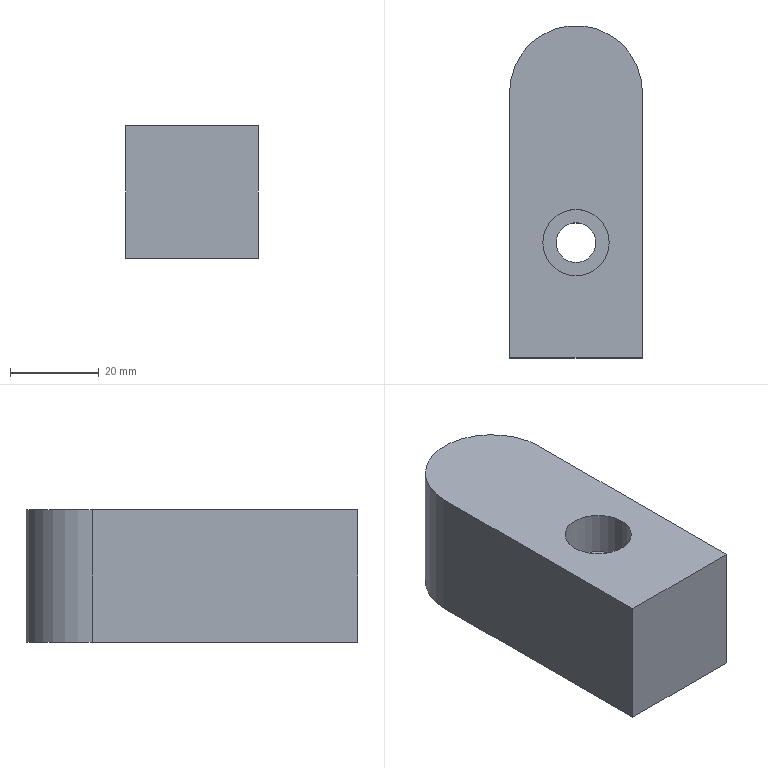Part | STEP file | 400v80 Tailstock Locating Pin | 1 solid | 11 faces | box 30 x 75 x 30 mm | volume 61563 mm3 | plane 6 | cylinder 5 | commonest cylinder face diameters 9 x2 15 x2 30 x1
STEP:
#1=CARTESIAN_POINT('',(-10.246,-122.222,0.));
#2=VERTEX_POINT('',#1);
#3=CARTESIAN_POINT('',(-19.246,-122.222,0.));
#4=VERTEX_POINT('',#3);
#5=CARTESIAN_POINT('',(-14.746,-122.222,0.));
#6=DIRECTION('',(0.,0.,-1.));
#7=DIRECTION('',(1.,0.,0.));
#8=AXIS2_PLACEMENT_3D('',#5,#6,#7);
#9=CIRCLE('',#8,4.5);
#10=EDGE_CURVE('',#2,#4,#9,.T.);
#11=ORIENTED_EDGE('',*,*,#10,.T.);
#12=CARTESIAN_POINT('',(-19.246,-122.222,20.));
#13=VERTEX_POINT('',#12);
#14=CARTESIAN_POINT('',(-19.246,-122.222,0.));
#15=DIRECTION('',(0.,0.,1.));
#16=VECTOR('',#15,1000.);
#17=LINE('',#14,#16);
#18=EDGE_CURVE('',#4,#13,#17,.T.);
#19=ORIENTED_EDGE('',*,*,#18,.T.);
#20=CARTESIAN_POINT('',(-10.246,-122.222,20.));
#21=VERTEX_POINT('',#20);
#22=CARTESIAN_POINT('',(-14.746,-122.222,20.));
#23=DIRECTION('',(0.,0.,-1.));
#24=DIRECTION('',(1.,0.,0.));
#25=AXIS2_PLACEMENT_3D('',#22,#23,#24);
#26=CIRCLE('',#25,4.5);
#27=EDGE_CURVE('',#21,#13,#26,.T.);
#28=ORIENTED_EDGE('',*,*,#27,.F.);
#29=CARTESIAN_POINT('',(-10.246,-122.222,0.));
#30=DIRECTION('',(0.,0.,1.));
#31=VECTOR('',#30,1000.);
#32=LINE('',#29,#31);
#33=EDGE_CURVE('',#2,#21,#32,.T.);
#34=ORIENTED_EDGE('',*,*,#33,.F.);
#35=EDGE_LOOP('',(#11,#19,#28,#34));
#36=FACE_OUTER_BOUND('',#35,.T.);
#37=CARTESIAN_POINT('',(-14.746,-122.222,0.));
#38=DIRECTION('',(0.,0.,1.));
#39=DIRECTION('',(1.,0.,0.));
#40=AXIS2_PLACEMENT_3D('',#37,#38,#39);
#41=CYLINDRICAL_SURFACE('',#40,4.5);
#42=ADVANCED_FACE('',(#36),#41,.F.);
#43=CARTESIAN_POINT('',(-22.246,-122.222,20.));
#44=VERTEX_POINT('',#43);
#45=CARTESIAN_POINT('',(-7.246,-122.222,20.));
#46=VERTEX_POINT('',#45);
#47=CARTESIAN_POINT('',(-14.746,-122.222,20.));
#48=DIRECTION('',(0.,0.,1.));
#49=DIRECTION('',(1.,0.,0.));
#50=AXIS2_PLACEMENT_3D('',#47,#48,#49);
#51=CIRCLE('',#50,7.5);
#52=EDGE_CURVE('',#44,#46,#51,.T.);
#53=ORIENTED_EDGE('',*,*,#52,.F.);
#54=CARTESIAN_POINT('',(-22.246,-122.222,30.));
#55=VERTEX_POINT('',#54);
#56=CARTESIAN_POINT('',(-22.246,-122.222,20.));
#57=DIRECTION('',(0.,0.,1.));
#58=VECTOR('',#57,1000.);
#59=LINE('',#56,#58);
#60=EDGE_CURVE('',#44,#55,#59,.T.);
#61=ORIENTED_EDGE('',*,*,#60,.T.);
#62=CARTESIAN_POINT('',(-7.246,-122.222,30.));
#63=VERTEX_POINT('',#62);
#64=CARTESIAN_POINT('',(-14.746,-122.222,30.));
#65=DIRECTION('',(0.,0.,-1.));
#66=DIRECTION('',(1.,0.,0.));
#67=AXIS2_PLACEMENT_3D('',#64,#65,#66);
#68=CIRCLE('',#67,7.5);
#69=EDGE_CURVE('',#63,#55,#68,.T.);
#70=ORIENTED_EDGE('',*,*,#69,.F.);
#71=CARTESIAN_POINT('',(-7.246,-122.222,20.));
#72=DIRECTION('',(0.,0.,1.));
#73=VECTOR('',#72,1000.);
#74=LINE('',#71,#73);
#75=EDGE_CURVE('',#46,#63,#74,.T.);
#76=ORIENTED_EDGE('',*,*,#75,.F.);
#77=EDGE_LOOP('',(#53,#61,#70,#76));
#78=FACE_OUTER_BOUND('',#77,.T.);
#79=CARTESIAN_POINT('',(-14.746,-122.222,20.));
#80=DIRECTION('',(0.,0.,1.));
#81=DIRECTION('',(1.,0.,0.));
#82=AXIS2_PLACEMENT_3D('',#79,#80,#81);
#83=CYLINDRICAL_SURFACE('',#82,7.5);
#84=ADVANCED_FACE('',(#78),#83,.F.);
#85=CARTESIAN_POINT('',(0.2545,-148.222,0.));
#86=VERTEX_POINT('',#85);
#87=CARTESIAN_POINT('',(0.2545,-88.222,0.));
#88=VERTEX_POINT('',#87);
#89=CARTESIAN_POINT('',(0.2545,-88.222,0.));
#90=DIRECTION('',(0.,1.,0.));
#91=VECTOR('',#90,1000.);
#92=LINE('',#89,#91);
#93=EDGE_CURVE('',#86,#88,#92,.T.);
#94=ORIENTED_EDGE('',*,*,#93,.F.);
#95=CARTESIAN_POINT('',(-29.746,-148.222,0.));
#96=VERTEX_POINT('',#95);
#97=CARTESIAN_POINT('',(-14.746,-148.222,0.));
#98=DIRECTION('',(1.,0.,0.));
#99=VECTOR('',#98,1000.);
#100=LINE('',#97,#99);
#101=EDGE_CURVE('',#96,#86,#100,.T.);
#102=ORIENTED_EDGE('',*,*,#101,.F.);
#103=CARTESIAN_POINT('',(-29.746,-88.222,0.));
#104=VERTEX_POINT('',#103);
#105=CARTESIAN_POINT('',(-29.746,-88.222,0.));
#106=DIRECTION('',(0.,-1.,0.));
#107=VECTOR('',#106,1000.);
#108=LINE('',#105,#107);
#109=EDGE_CURVE('',#104,#96,#108,.T.);
#110=ORIENTED_EDGE('',*,*,#109,.F.);
#111=CARTESIAN_POINT('',(-14.746,-88.222,0.));
#112=DIRECTION('',(0.,0.,1.));
#113=DIRECTION('',(-1.,0.,0.));
#114=AXIS2_PLACEMENT_3D('',#111,#112,#113);
#115=CIRCLE('',#114,15.);
#116=EDGE_CURVE('',#88,#104,#115,.T.);
#117=ORIENTED_EDGE('',*,*,#116,.F.);
#118=EDGE_LOOP('',(#94,#102,#110,#117));
#119=FACE_OUTER_BOUND('',#118,.T.);
#120=ORIENTED_EDGE('',*,*,#10,.F.);
#121=CARTESIAN_POINT('',(-14.746,-122.222,0.));
#122=DIRECTION('',(0.,0.,-1.));
#123=DIRECTION('',(1.,0.,0.));
#124=AXIS2_PLACEMENT_3D('',#121,#122,#123);
#125=CIRCLE('',#124,4.5);
#126=EDGE_CURVE('',#4,#2,#125,.T.);
#127=ORIENTED_EDGE('',*,*,#126,.F.);
#128=EDGE_LOOP('',(#120,#127));
#129=FACE_BOUND('',#128,.T.);
#130=CARTESIAN_POINT('',(-14.746,-88.222,0.));
#131=DIRECTION('',(0.,0.,1.));
#132=DIRECTION('',(1.,0.,0.));
#133=AXIS2_PLACEMENT_3D('',#130,#131,#132);
#134=PLANE('',#133);
#135=ADVANCED_FACE('',(#119,#129),#134,.F.);
#136=CARTESIAN_POINT('',(-29.746,-88.222,30.));
#137=VERTEX_POINT('',#136);
#138=CARTESIAN_POINT('',(0.2545,-88.222,30.));
#139=VERTEX_POINT('',#138);
#140=CARTESIAN_POINT('',(-14.746,-88.222,30.));
#141=DIRECTION('',(0.,0.,-1.));
#142=DIRECTION('',(-1.,0.,0.));
#143=AXIS2_PLACEMENT_3D('',#140,#141,#142);
#144=CIRCLE('',#143,15.);
#145=EDGE_CURVE('',#137,#139,#144,.T.);
#146=ORIENTED_EDGE('',*,*,#145,.T.);
#147=CARTESIAN_POINT('',(0.2545,-88.222,30.));
#148=DIRECTION('',(0.,0.,-1.));
#149=VECTOR('',#148,1000.);
#150=LINE('',#147,#149);
#151=EDGE_CURVE('',#139,#88,#150,.T.);
#152=ORIENTED_EDGE('',*,*,#151,.T.);
#153=ORIENTED_EDGE('',*,*,#116,.T.);
#154=CARTESIAN_POINT('',(-29.746,-88.222,30.));
#155=DIRECTION('',(0.,0.,1.));
#156=VECTOR('',#155,1000.);
#157=LINE('',#154,#156);
#158=EDGE_CURVE('',#104,#137,#157,.T.);
#159=ORIENTED_EDGE('',*,*,#158,.T.);
#160=EDGE_LOOP('',(#146,#152,#153,#159));
#161=FACE_OUTER_BOUND('',#160,.T.);
#162=CARTESIAN_POINT('',(-14.746,-88.222,30.));
#163=DIRECTION('',(0.,0.,-1.));
#164=DIRECTION('',(-1.,0.,0.));
#165=AXIS2_PLACEMENT_3D('',#162,#163,#164);
#166=CYLINDRICAL_SURFACE('',#165,15.);
#167=ADVANCED_FACE('',(#161),#166,.T.);
#168=ORIENTED_EDGE('',*,*,#151,.F.);
#169=CARTESIAN_POINT('',(0.2545,-148.222,30.));
#170=VERTEX_POINT('',#169);
#171=CARTESIAN_POINT('',(0.2545,-88.222,30.));
#172=DIRECTION('',(0.,1.,0.));
#173=VECTOR('',#172,1000.);
#174=LINE('',#171,#173);
#175=EDGE_CURVE('',#170,#139,#174,.T.);
#176=ORIENTED_EDGE('',*,*,#175,.F.);
#177=CARTESIAN_POINT('',(0.2545,-148.222,30.));
#178=DIRECTION('',(0.,0.,1.));
#179=VECTOR('',#178,1000.);
#180=LINE('',#177,#179);
#181=EDGE_CURVE('',#86,#170,#180,.T.);
#182=ORIENTED_EDGE('',*,*,#181,.F.);
#183=ORIENTED_EDGE('',*,*,#93,.T.);
#184=EDGE_LOOP('',(#168,#176,#182,#183));
#185=FACE_OUTER_BOUND('',#184,.T.);
#186=CARTESIAN_POINT('',(0.2545,-88.222,30.));
#187=DIRECTION('',(-1.,0.,0.));
#188=DIRECTION('',(0.,-1.,0.));
#189=AXIS2_PLACEMENT_3D('',#186,#187,#188);
#190=PLANE('',#189);
#191=ADVANCED_FACE('',(#185),#190,.F.);
#192=ORIENTED_EDGE('',*,*,#181,.T.);
#193=CARTESIAN_POINT('',(-29.746,-148.222,30.));
#194=VERTEX_POINT('',#193);
#195=CARTESIAN_POINT('',(-29.746,-148.222,30.));
#196=DIRECTION('',(1.,0.,0.));
#197=VECTOR('',#196,1000.);
#198=LINE('',#195,#197);
#199=EDGE_CURVE('',#194,#170,#198,.T.);
#200=ORIENTED_EDGE('',*,*,#199,.F.);
#201=CARTESIAN_POINT('',(-29.746,-148.222,30.));
#202=DIRECTION('',(0.,0.,1.));
#203=VECTOR('',#202,1000.);
#204=LINE('',#201,#203);
#205=EDGE_CURVE('',#96,#194,#204,.T.);
#206=ORIENTED_EDGE('',*,*,#205,.F.);
#207=ORIENTED_EDGE('',*,*,#101,.T.);
#208=EDGE_LOOP('',(#192,#200,#206,#207));
#209=FACE_OUTER_BOUND('',#208,.T.);
#210=CARTESIAN_POINT('',(-29.746,-148.222,30.));
#211=DIRECTION('',(0.,1.,0.));
#212=DIRECTION('',(0.,0.,1.));
#213=AXIS2_PLACEMENT_3D('',#210,#211,#212);
#214=PLANE('',#213);
#215=ADVANCED_FACE('',(#209),#214,.F.);
#216=ORIENTED_EDGE('',*,*,#205,.T.);
#217=CARTESIAN_POINT('',(-29.746,-88.222,30.));
#218=DIRECTION('',(0.,-1.,0.));
#219=VECTOR('',#218,1000.);
#220=LINE('',#217,#219);
#221=EDGE_CURVE('',#137,#194,#220,.T.);
#222=ORIENTED_EDGE('',*,*,#221,.F.);
#223=ORIENTED_EDGE('',*,*,#158,.F.);
#224=ORIENTED_EDGE('',*,*,#109,.T.);
#225=EDGE_LOOP('',(#216,#222,#223,#224));
#226=FACE_OUTER_BOUND('',#225,.T.);
#227=CARTESIAN_POINT('',(-29.746,-88.222,30.));
#228=DIRECTION('',(1.,0.,0.));
#229=DIRECTION('',(0.,1.,0.));
#230=AXIS2_PLACEMENT_3D('',#227,#228,#229);
#231=PLANE('',#230);
#232=ADVANCED_FACE('',(#226),#231,.F.);
#233=ORIENTED_EDGE('',*,*,#18,.F.);
#234=ORIENTED_EDGE('',*,*,#126,.T.);
#235=ORIENTED_EDGE('',*,*,#33,.T.);
#236=CARTESIAN_POINT('',(-14.746,-122.222,20.));
#237=DIRECTION('',(0.,0.,-1.));
#238=DIRECTION('',(1.,0.,0.));
#239=AXIS2_PLACEMENT_3D('',#236,#237,#238);
#240=CIRCLE('',#239,4.5);
#241=EDGE_CURVE('',#13,#21,#240,.T.);
#242=ORIENTED_EDGE('',*,*,#241,.F.);
#243=EDGE_LOOP('',(#233,#234,#235,#242));
#244=FACE_OUTER_BOUND('',#243,.T.);
#245=CARTESIAN_POINT('',(-14.746,-122.222,0.));
#246=DIRECTION('',(0.,0.,1.));
#247=DIRECTION('',(1.,0.,0.));
#248=AXIS2_PLACEMENT_3D('',#245,#246,#247);
#249=CYLINDRICAL_SURFACE('',#248,4.5);
#250=ADVANCED_FACE('',(#244),#249,.F.);
#251=ORIENTED_EDGE('',*,*,#199,.T.);
#252=ORIENTED_EDGE('',*,*,#175,.T.);
#253=ORIENTED_EDGE('',*,*,#145,.F.);
#254=ORIENTED_EDGE('',*,*,#221,.T.);
#255=EDGE_LOOP('',(#251,#252,#253,#254));
#256=FACE_OUTER_BOUND('',#255,.T.);
#257=ORIENTED_EDGE('',*,*,#69,.T.);
#258=CARTESIAN_POINT('',(-14.746,-122.222,30.));
#259=DIRECTION('',(0.,0.,-1.));
#260=DIRECTION('',(1.,0.,0.));
#261=AXIS2_PLACEMENT_3D('',#258,#259,#260);
#262=CIRCLE('',#261,7.5);
#263=EDGE_CURVE('',#55,#63,#262,.T.);
#264=ORIENTED_EDGE('',*,*,#263,.T.);
#265=EDGE_LOOP('',(#257,#264));
#266=FACE_BOUND('',#265,.T.);
#267=CARTESIAN_POINT('',(-14.746,-88.222,30.));
#268=DIRECTION('',(0.,0.,1.));
#269=DIRECTION('',(1.,0.,0.));
#270=AXIS2_PLACEMENT_3D('',#267,#268,#269);
#271=PLANE('',#270);
#272=ADVANCED_FACE('',(#256,#266),#271,.T.);
#273=ORIENTED_EDGE('',*,*,#27,.T.);
#274=ORIENTED_EDGE('',*,*,#241,.T.);
#275=EDGE_LOOP('',(#273,#274));
#276=FACE_BOUND('',#275,.T.);
#277=CARTESIAN_POINT('',(-14.746,-122.222,20.));
#278=DIRECTION('',(0.,0.,1.));
#279=DIRECTION('',(1.,0.,0.));
#280=AXIS2_PLACEMENT_3D('',#277,#278,#279);
#281=CIRCLE('',#280,7.5);
#282=EDGE_CURVE('',#46,#44,#281,.T.);
#283=ORIENTED_EDGE('',*,*,#282,.T.);
#284=ORIENTED_EDGE('',*,*,#52,.T.);
#285=EDGE_LOOP('',(#283,#284));
#286=FACE_OUTER_BOUND('',#285,.T.);
#287=CARTESIAN_POINT('',(-14.746,-122.222,20.));
#288=DIRECTION('',(0.,0.,1.));
#289=DIRECTION('',(1.,0.,0.));
#290=AXIS2_PLACEMENT_3D('',#287,#288,#289);
#291=PLANE('',#290);
#292=ADVANCED_FACE('',(#276,#286),#291,.T.);
#293=ORIENTED_EDGE('',*,*,#60,.F.);
#294=ORIENTED_EDGE('',*,*,#282,.F.);
#295=ORIENTED_EDGE('',*,*,#75,.T.);
#296=ORIENTED_EDGE('',*,*,#263,.F.);
#297=EDGE_LOOP('',(#293,#294,#295,#296));
#298=FACE_OUTER_BOUND('',#297,.T.);
#299=CARTESIAN_POINT('',(-14.746,-122.222,20.));
#300=DIRECTION('',(0.,0.,1.));
#301=DIRECTION('',(1.,0.,0.));
#302=AXIS2_PLACEMENT_3D('',#299,#300,#301);
#303=CYLINDRICAL_SURFACE('',#302,7.5);
#304=ADVANCED_FACE('',(#298),#303,.F.);
#305=CLOSED_SHELL('',(#42,#84,#135,#167,#191,#215,#232,#250,#272,#292,#304));
#306=MANIFOLD_SOLID_BREP('',#305);
#307=CARTESIAN_POINT('',(0.,0.,0.));
#308=DIRECTION('',(0.,0.,1.));
#309=DIRECTION('',(1.,0.,0.));
#310=AXIS2_PLACEMENT_3D('',#307,#308,#309);
#311=(LENGTH_UNIT()NAMED_UNIT(*)SI_UNIT(.MILLI.,.METRE.));
#312=UNCERTAINTY_MEASURE_WITH_UNIT(LENGTH_MEASURE(0.00001),#311,'','');
#313=(NAMED_UNIT(*)PLANE_ANGLE_UNIT()SI_UNIT($,.RADIAN.));
#314=(NAMED_UNIT(*)SI_UNIT($,.STERADIAN.)SOLID_ANGLE_UNIT());
#315=(GEOMETRIC_REPRESENTATION_CONTEXT(3)GLOBAL_UNCERTAINTY_ASSIGNED_CONTEXT((#312))GLOBAL_UNIT_ASSIGNED_CONTEXT((#311,#313,#314))REPRESENTATION_CONTEXT('',''));
#316=ADVANCED_BREP_SHAPE_REPRESENTATION('',(#306,#310),#315);